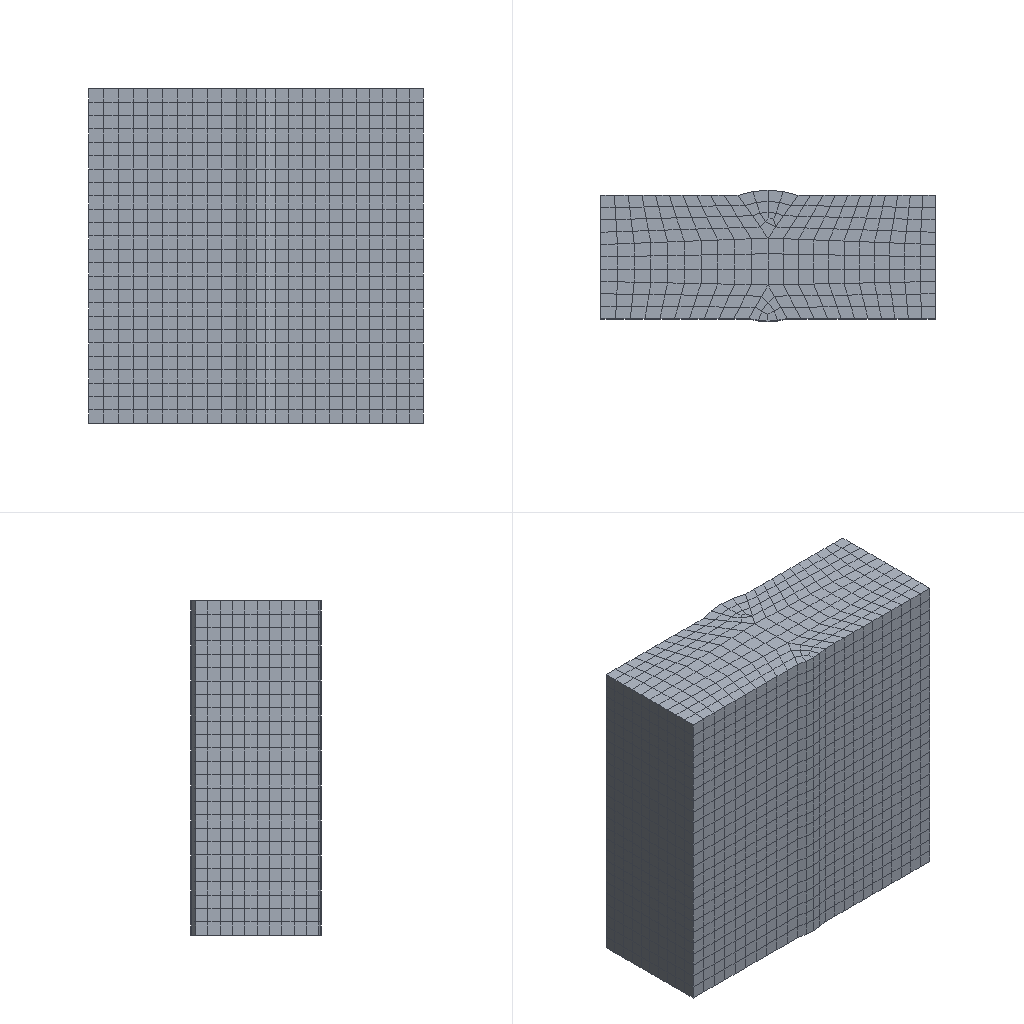Simulation study | abaqus
Set-up summary:
category,name,step,type,value,unit,region
solver,abaqus
solver,version,,,Abaqus/Standard 3DEXPERIENCE R2017x
units,not stated in the deck,,not stated
analysis,deck,,coupled temperature-displacement,coupled temperature-displacement
load_step,kill,kill,coupled temperature-displacement,nlgeom=True
load_step,r1,r1,coupled temperature-displacement,nlgeom=True
load_step,w1,w1,coupled temperature-displacement,nlgeom=True
load_step,r2,r2,coupled temperature-displacement,nlgeom=True
load_step,w2,w2,coupled temperature-displacement,nlgeom=True
load_step,r3,r3,coupled temperature-displacement,nlgeom=True
load_step,w3,w3,coupled temperature-displacement,nlgeom=True
load_step,cooling,cooling,coupled temperature-displacement,nlgeom=True
contact,interactions,,,general=0 pairs=0 ties=0
load_step,requested,,,8
mesh,nodes,,,6968
mesh,elements,,,5800
element_type,C3D8RT,,solid,5800
load,load commands in deck,,count,2
bc,support commands in deck,,count,2
material,MATERIAL-1,,in results
check,setup vs results,,match,"per instance, exact: element labels, types and connectivity; labels of the nodes the elements use; coordinates not compared"
Results summary:
result,step,,completed,increments=1 time=1e-08/1e-08
result,step,,completed,increments=1 time=1e-08/1e-08
result,step,,completed,increments=164 time=6.024/6.024
result,step,,completed,increments=1 time=1e-08/1e-08
result,step,,completed,increments=145 time=3.75/3.75
result,step,,completed,increments=1 time=1e-08/1e-08
result,step,,completed,increments=81 time=3.75/3.75
result,step,,completed,increments=29 time=1000.0/1000.0
result,analysis,,,"coupled temperature-displacement, steady state"
result,last_loadstep,,,8
result,analysis steps,,count,8
result,primary field,,,"U, NT11"
result,reaction total,,FX,-0.004364,model units
result,reaction total,,FY,-0.004241,model units
result,reaction total,,FZ,0.1133,model units